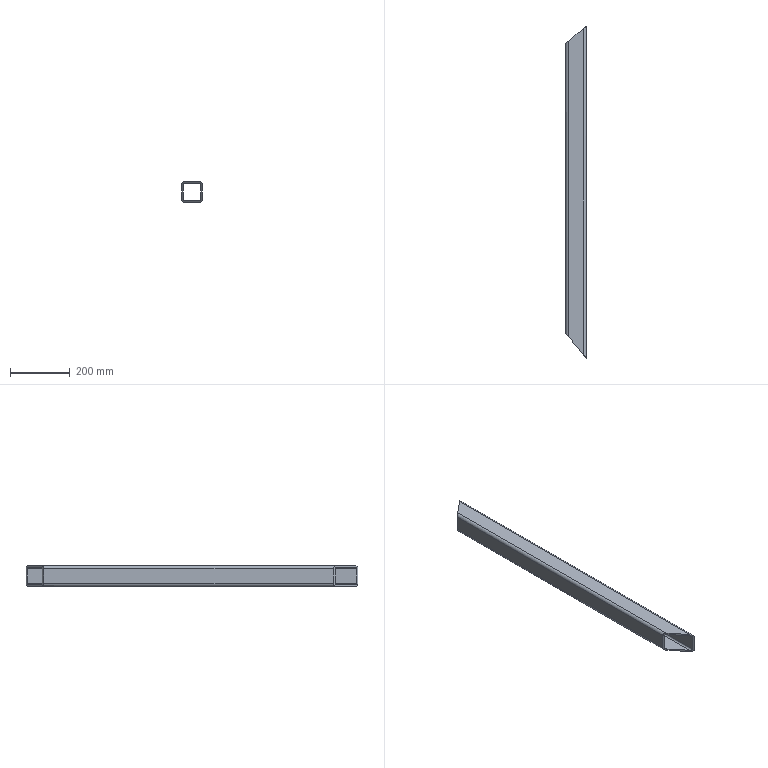Part | SolidWorks | features ICE 1, WeldMemberFeat 1, WeldmentFeature 1 | 1 solid | 18 faces | box 70 x 1116 x 70 mm | volume 1291200 mm3 | plane 10 | cylinder 8 | commonest cylinder face diameters 10 x4 20 x4
STEP:
#1=CARTESIAN_POINT('',(35.,0.,25.));
#2=VERTEX_POINT('',#1);
#3=CARTESIAN_POINT('',(35.,0.,-25.));
#4=VERTEX_POINT('',#3);
#5=CARTESIAN_POINT('',(35.,0.,-25.));
#6=DIRECTION('',(0.,0.,-1.));
#7=VECTOR('',#6,1000.);
#8=LINE('',#5,#7);
#9=EDGE_CURVE('',#2,#4,#8,.T.);
#10=ORIENTED_EDGE('',*,*,#9,.T.);
#11=CARTESIAN_POINT('',(35.,1116.,-25.));
#12=VERTEX_POINT('',#11);
#13=CARTESIAN_POINT('',(35.,1116.,-25.));
#14=DIRECTION('',(0.,-1.,0.));
#15=VECTOR('',#14,1000.);
#16=LINE('',#13,#15);
#17=EDGE_CURVE('',#12,#4,#16,.T.);
#18=ORIENTED_EDGE('',*,*,#17,.F.);
#19=CARTESIAN_POINT('',(35.,1116.,25.));
#20=VERTEX_POINT('',#19);
#21=CARTESIAN_POINT('',(35.,1116.,-25.));
#22=DIRECTION('',(0.,0.,-1.));
#23=VECTOR('',#22,1000.);
#24=LINE('',#21,#23);
#25=EDGE_CURVE('',#20,#12,#24,.T.);
#26=ORIENTED_EDGE('',*,*,#25,.F.);
#27=CARTESIAN_POINT('',(35.,1116.,25.));
#28=DIRECTION('',(0.,-1.,0.));
#29=VECTOR('',#28,1000.);
#30=LINE('',#27,#29);
#31=EDGE_CURVE('',#20,#2,#30,.T.);
#32=ORIENTED_EDGE('',*,*,#31,.T.);
#33=EDGE_LOOP('',(#10,#18,#26,#32));
#34=FACE_OUTER_BOUND('',#33,.T.);
#35=CARTESIAN_POINT('',(35.,1116.,-25.));
#36=DIRECTION('',(-1.,0.,0.));
#37=DIRECTION('',(0.,0.,1.));
#38=AXIS2_PLACEMENT_3D('',#35,#36,#37);
#39=PLANE('',#38);
#40=ADVANCED_FACE('',(#34),#39,.F.);
#41=CARTESIAN_POINT('',(-35.,1056.964,25.));
#42=VERTEX_POINT('',#41);
#43=CARTESIAN_POINT('',(-35.,83.,25.));
#44=VERTEX_POINT('',#43);
#45=CARTESIAN_POINT('',(-35.,1116.,25.));
#46=DIRECTION('',(0.,-1.,0.));
#47=VECTOR('',#46,1000.);
#48=LINE('',#45,#47);
#49=EDGE_CURVE('',#42,#44,#48,.T.);
#50=ORIENTED_EDGE('',*,*,#49,.F.);
#51=CARTESIAN_POINT('',(-35.,1056.964,-25.));
#52=VERTEX_POINT('',#51);
#53=CARTESIAN_POINT('',(-35.,1056.964,-35.));
#54=DIRECTION('',(0.,0.,1.));
#55=VECTOR('',#54,1000.);
#56=LINE('',#53,#55);
#57=EDGE_CURVE('',#52,#42,#56,.T.);
#58=ORIENTED_EDGE('',*,*,#57,.F.);
#59=CARTESIAN_POINT('',(-35.,83.,-25.));
#60=VERTEX_POINT('',#59);
#61=CARTESIAN_POINT('',(-35.,1116.,-25.));
#62=DIRECTION('',(0.,-1.,0.));
#63=VECTOR('',#62,1000.);
#64=LINE('',#61,#63);
#65=EDGE_CURVE('',#52,#60,#64,.T.);
#66=ORIENTED_EDGE('',*,*,#65,.T.);
#67=CARTESIAN_POINT('',(-35.,83.,-35.));
#68=DIRECTION('',(0.,0.,1.));
#69=VECTOR('',#68,1000.);
#70=LINE('',#67,#69);
#71=EDGE_CURVE('',#60,#44,#70,.T.);
#72=ORIENTED_EDGE('',*,*,#71,.T.);
#73=EDGE_LOOP('',(#50,#58,#66,#72));
#74=FACE_OUTER_BOUND('',#73,.T.);
#75=CARTESIAN_POINT('',(-35.,1116.,25.));
#76=DIRECTION('',(1.,0.,0.));
#77=DIRECTION('',(0.,0.,-1.));
#78=AXIS2_PLACEMENT_3D('',#75,#76,#77);
#79=PLANE('',#78);
#80=ADVANCED_FACE('',(#74),#79,.F.);
#81=ORIENTED_EDGE('',*,*,#65,.F.);
#82=CARTESIAN_POINT('',(-25.,1065.398,-35.));
#83=VERTEX_POINT('',#82);
#84=CARTESIAN_POINT('',(-35.,1056.964,-25.));
#85=CARTESIAN_POINT('',(-35.,1056.964,-30.858));
#86=CARTESIAN_POINT('',(-30.858,1060.457,-35.));
#87=CARTESIAN_POINT('',(-25.,1065.398,-35.));
#88=(BOUNDED_CURVE()B_SPLINE_CURVE(3,(#84,#85,#86,#87),.UNSPECIFIED.,.F.,.F.)B_SPLINE_CURVE_WITH_KNOTS((4,4),(0.,1.571),.UNSPECIFIED.)CURVE()GEOMETRIC_REPRESENTATION_ITEM()RATIONAL_B_SPLINE_CURVE((1.,0.8047,0.8047,1.))REPRESENTATION_ITEM(''));
#89=EDGE_CURVE('',#52,#83,#88,.T.);
#90=ORIENTED_EDGE('',*,*,#89,.T.);
#91=CARTESIAN_POINT('',(-25.,71.143,-35.));
#92=VERTEX_POINT('',#91);
#93=CARTESIAN_POINT('',(-25.,1116.,-35.));
#94=DIRECTION('',(0.,-1.,0.));
#95=VECTOR('',#94,1000.);
#96=LINE('',#93,#95);
#97=EDGE_CURVE('',#83,#92,#96,.T.);
#98=ORIENTED_EDGE('',*,*,#97,.T.);
#99=CARTESIAN_POINT('',(-25.,71.143,-35.));
#100=CARTESIAN_POINT('',(-30.858,78.089,-35.));
#101=CARTESIAN_POINT('',(-35.,83.,-30.858));
#102=CARTESIAN_POINT('',(-35.,83.,-25.));
#103=(BOUNDED_CURVE()B_SPLINE_CURVE(3,(#99,#100,#101,#102),.UNSPECIFIED.,.F.,.F.)B_SPLINE_CURVE_WITH_KNOTS((4,4),(1.571,3.142),.UNSPECIFIED.)CURVE()GEOMETRIC_REPRESENTATION_ITEM()RATIONAL_B_SPLINE_CURVE((1.,0.8047,0.8047,1.))REPRESENTATION_ITEM(''));
#104=EDGE_CURVE('',#92,#60,#103,.T.);
#105=ORIENTED_EDGE('',*,*,#104,.T.);
#106=EDGE_LOOP('',(#81,#90,#98,#105));
#107=FACE_OUTER_BOUND('',#106,.T.);
#108=CARTESIAN_POINT('',(-25.,1116.,-25.));
#109=DIRECTION('',(0.,-1.,0.));
#110=DIRECTION('',(0.,0.,-1.));
#111=AXIS2_PLACEMENT_3D('',#108,#109,#110);
#112=CYLINDRICAL_SURFACE('',#111,10.);
#113=ADVANCED_FACE('',(#107),#112,.T.);
#114=ORIENTED_EDGE('',*,*,#97,.F.);
#115=CARTESIAN_POINT('',(25.,1107.566,-35.));
#116=VERTEX_POINT('',#115);
#117=CARTESIAN_POINT('',(35.,1116.,-35.));
#118=DIRECTION('',(0.7644,0.6447,0.));
#119=VECTOR('',#118,1000.);
#120=LINE('',#117,#119);
#121=EDGE_CURVE('',#83,#116,#120,.T.);
#122=ORIENTED_EDGE('',*,*,#121,.T.);
#123=CARTESIAN_POINT('',(25.,11.857,-35.));
#124=VERTEX_POINT('',#123);
#125=CARTESIAN_POINT('',(25.,1116.,-35.));
#126=DIRECTION('',(0.,-1.,0.));
#127=VECTOR('',#126,1000.);
#128=LINE('',#125,#127);
#129=EDGE_CURVE('',#116,#124,#128,.T.);
#130=ORIENTED_EDGE('',*,*,#129,.T.);
#131=CARTESIAN_POINT('',(-35.,83.,-35.));
#132=DIRECTION('',(-0.6447,0.7644,0.));
#133=VECTOR('',#132,1000.);
#134=LINE('',#131,#133);
#135=EDGE_CURVE('',#124,#92,#134,.T.);
#136=ORIENTED_EDGE('',*,*,#135,.T.);
#137=EDGE_LOOP('',(#114,#122,#130,#136));
#138=FACE_OUTER_BOUND('',#137,.T.);
#139=CARTESIAN_POINT('',(25.,1116.,-35.));
#140=DIRECTION('',(0.,0.,1.));
#141=DIRECTION('',(1.,0.,0.));
#142=AXIS2_PLACEMENT_3D('',#139,#140,#141);
#143=PLANE('',#142);
#144=ADVANCED_FACE('',(#138),#143,.F.);
#145=ORIENTED_EDGE('',*,*,#129,.F.);
#146=CARTESIAN_POINT('',(25.,1107.566,-35.));
#147=CARTESIAN_POINT('',(30.858,1112.507,-35.));
#148=CARTESIAN_POINT('',(35.,1116.,-30.858));
#149=CARTESIAN_POINT('',(35.,1116.,-25.));
#150=(BOUNDED_CURVE()B_SPLINE_CURVE(3,(#146,#147,#148,#149),.UNSPECIFIED.,.F.,.F.)B_SPLINE_CURVE_WITH_KNOTS((4,4),(1.571,3.142),.UNSPECIFIED.)CURVE()GEOMETRIC_REPRESENTATION_ITEM()RATIONAL_B_SPLINE_CURVE((1.,0.8047,0.8047,1.))REPRESENTATION_ITEM(''));
#151=EDGE_CURVE('',#116,#12,#150,.T.);
#152=ORIENTED_EDGE('',*,*,#151,.T.);
#153=ORIENTED_EDGE('',*,*,#17,.T.);
#154=CARTESIAN_POINT('',(35.,0.,-25.));
#155=CARTESIAN_POINT('',(35.,0.,-30.858));
#156=CARTESIAN_POINT('',(30.858,4.911,-35.));
#157=CARTESIAN_POINT('',(25.,11.857,-35.));
#158=(BOUNDED_CURVE()B_SPLINE_CURVE(3,(#154,#155,#156,#157),.UNSPECIFIED.,.F.,.F.)B_SPLINE_CURVE_WITH_KNOTS((4,4),(0.,1.571),.UNSPECIFIED.)CURVE()GEOMETRIC_REPRESENTATION_ITEM()RATIONAL_B_SPLINE_CURVE((1.,0.8047,0.8047,1.))REPRESENTATION_ITEM(''));
#159=EDGE_CURVE('',#4,#124,#158,.T.);
#160=ORIENTED_EDGE('',*,*,#159,.T.);
#161=EDGE_LOOP('',(#145,#152,#153,#160));
#162=FACE_OUTER_BOUND('',#161,.T.);
#163=CARTESIAN_POINT('',(25.,1116.,-25.));
#164=DIRECTION('',(0.,-1.,0.));
#165=DIRECTION('',(0.,0.,-1.));
#166=AXIS2_PLACEMENT_3D('',#163,#164,#165);
#167=CYLINDRICAL_SURFACE('',#166,10.);
#168=ADVANCED_FACE('',(#162),#167,.T.);
#169=ORIENTED_EDGE('',*,*,#31,.F.);
#170=CARTESIAN_POINT('',(25.,1107.566,35.));
#171=VERTEX_POINT('',#170);
#172=CARTESIAN_POINT('',(35.,1116.,25.));
#173=CARTESIAN_POINT('',(35.,1116.,30.858));
#174=CARTESIAN_POINT('',(30.858,1112.507,35.));
#175=CARTESIAN_POINT('',(25.,1107.566,35.));
#176=(BOUNDED_CURVE()B_SPLINE_CURVE(3,(#172,#173,#174,#175),.UNSPECIFIED.,.F.,.F.)B_SPLINE_CURVE_WITH_KNOTS((4,4),(3.142,4.712),.UNSPECIFIED.)CURVE()GEOMETRIC_REPRESENTATION_ITEM()RATIONAL_B_SPLINE_CURVE((1.,0.8047,0.8047,1.))REPRESENTATION_ITEM(''));
#177=EDGE_CURVE('',#20,#171,#176,.T.);
#178=ORIENTED_EDGE('',*,*,#177,.T.);
#179=CARTESIAN_POINT('',(25.,11.857,35.));
#180=VERTEX_POINT('',#179);
#181=CARTESIAN_POINT('',(25.,1116.,35.));
#182=DIRECTION('',(0.,-1.,0.));
#183=VECTOR('',#182,1000.);
#184=LINE('',#181,#183);
#185=EDGE_CURVE('',#171,#180,#184,.T.);
#186=ORIENTED_EDGE('',*,*,#185,.T.);
#187=CARTESIAN_POINT('',(25.,11.857,35.));
#188=CARTESIAN_POINT('',(30.858,4.911,35.));
#189=CARTESIAN_POINT('',(35.,0.,30.858));
#190=CARTESIAN_POINT('',(35.,0.,25.));
#191=(BOUNDED_CURVE()B_SPLINE_CURVE(3,(#187,#188,#189,#190),.UNSPECIFIED.,.F.,.F.)B_SPLINE_CURVE_WITH_KNOTS((4,4),(4.712,6.283),.UNSPECIFIED.)CURVE()GEOMETRIC_REPRESENTATION_ITEM()RATIONAL_B_SPLINE_CURVE((1.,0.8047,0.8047,1.))REPRESENTATION_ITEM(''));
#192=EDGE_CURVE('',#180,#2,#191,.T.);
#193=ORIENTED_EDGE('',*,*,#192,.T.);
#194=EDGE_LOOP('',(#169,#178,#186,#193));
#195=FACE_OUTER_BOUND('',#194,.T.);
#196=CARTESIAN_POINT('',(25.,1116.,25.));
#197=DIRECTION('',(0.,-1.,0.));
#198=DIRECTION('',(0.,0.,-1.));
#199=AXIS2_PLACEMENT_3D('',#196,#197,#198);
#200=CYLINDRICAL_SURFACE('',#199,10.);
#201=ADVANCED_FACE('',(#195),#200,.T.);
#202=ORIENTED_EDGE('',*,*,#185,.F.);
#203=CARTESIAN_POINT('',(-25.,1065.398,35.));
#204=VERTEX_POINT('',#203);
#205=CARTESIAN_POINT('',(-0.0615,1086.43,35.));
#206=DIRECTION('',(-0.7644,-0.6447,0.));
#207=VECTOR('',#206,1000.);
#208=LINE('',#205,#207);
#209=EDGE_CURVE('',#171,#204,#208,.T.);
#210=ORIENTED_EDGE('',*,*,#209,.T.);
#211=CARTESIAN_POINT('',(-25.,71.143,35.));
#212=VERTEX_POINT('',#211);
#213=CARTESIAN_POINT('',(-25.,1116.,35.));
#214=DIRECTION('',(0.,-1.,0.));
#215=VECTOR('',#214,1000.);
#216=LINE('',#213,#215);
#217=EDGE_CURVE('',#204,#212,#216,.T.);
#218=ORIENTED_EDGE('',*,*,#217,.T.);
#219=CARTESIAN_POINT('',(-539.939,681.714,35.));
#220=DIRECTION('',(0.6447,-0.7644,0.));
#221=VECTOR('',#220,1000.);
#222=LINE('',#219,#221);
#223=EDGE_CURVE('',#212,#180,#222,.T.);
#224=ORIENTED_EDGE('',*,*,#223,.T.);
#225=EDGE_LOOP('',(#202,#210,#218,#224));
#226=FACE_OUTER_BOUND('',#225,.T.);
#227=CARTESIAN_POINT('',(-25.,1116.,35.));
#228=DIRECTION('',(0.,0.,-1.));
#229=DIRECTION('',(-1.,0.,0.));
#230=AXIS2_PLACEMENT_3D('',#227,#228,#229);
#231=PLANE('',#230);
#232=ADVANCED_FACE('',(#226),#231,.F.);
#233=ORIENTED_EDGE('',*,*,#217,.F.);
#234=CARTESIAN_POINT('',(-25.,1065.398,35.));
#235=CARTESIAN_POINT('',(-30.858,1060.457,35.));
#236=CARTESIAN_POINT('',(-35.,1056.964,30.858));
#237=CARTESIAN_POINT('',(-35.,1056.964,25.));
#238=(BOUNDED_CURVE()B_SPLINE_CURVE(3,(#234,#235,#236,#237),.UNSPECIFIED.,.F.,.F.)B_SPLINE_CURVE_WITH_KNOTS((4,4),(4.712,6.283),.UNSPECIFIED.)CURVE()GEOMETRIC_REPRESENTATION_ITEM()RATIONAL_B_SPLINE_CURVE((1.,0.8047,0.8047,1.))REPRESENTATION_ITEM(''));
#239=EDGE_CURVE('',#204,#42,#238,.T.);
#240=ORIENTED_EDGE('',*,*,#239,.T.);
#241=ORIENTED_EDGE('',*,*,#49,.T.);
#242=CARTESIAN_POINT('',(-35.,83.,25.));
#243=CARTESIAN_POINT('',(-35.,83.,30.858));
#244=CARTESIAN_POINT('',(-30.858,78.089,35.));
#245=CARTESIAN_POINT('',(-25.,71.143,35.));
#246=(BOUNDED_CURVE()B_SPLINE_CURVE(3,(#242,#243,#244,#245),.UNSPECIFIED.,.F.,.F.)B_SPLINE_CURVE_WITH_KNOTS((4,4),(3.142,4.712),.UNSPECIFIED.)CURVE()GEOMETRIC_REPRESENTATION_ITEM()RATIONAL_B_SPLINE_CURVE((1.,0.8047,0.8047,1.))REPRESENTATION_ITEM(''));
#247=EDGE_CURVE('',#44,#212,#246,.T.);
#248=ORIENTED_EDGE('',*,*,#247,.T.);
#249=EDGE_LOOP('',(#233,#240,#241,#248));
#250=FACE_OUTER_BOUND('',#249,.T.);
#251=CARTESIAN_POINT('',(-25.,1116.,25.));
#252=DIRECTION('',(0.,-1.,0.));
#253=DIRECTION('',(0.,0.,-1.));
#254=AXIS2_PLACEMENT_3D('',#251,#252,#253);
#255=CYLINDRICAL_SURFACE('',#254,10.);
#256=ADVANCED_FACE('',(#250),#255,.T.);
#257=CARTESIAN_POINT('',(25.,11.857,30.));
#258=VERTEX_POINT('',#257);
#259=CARTESIAN_POINT('',(30.,5.929,25.));
#260=VERTEX_POINT('',#259);
#261=CARTESIAN_POINT('',(25.,11.857,30.));
#262=CARTESIAN_POINT('',(27.929,8.384,30.));
#263=CARTESIAN_POINT('',(30.,5.929,27.929));
#264=CARTESIAN_POINT('',(30.,5.929,25.));
#265=(BOUNDED_CURVE()B_SPLINE_CURVE(3,(#261,#262,#263,#264),.UNSPECIFIED.,.F.,.T.)B_SPLINE_CURVE_WITH_KNOTS((4,4),(4.712,6.283),.UNSPECIFIED.)CURVE()GEOMETRIC_REPRESENTATION_ITEM()RATIONAL_B_SPLINE_CURVE((1.,0.8047,0.8047,1.))REPRESENTATION_ITEM(''));
#266=EDGE_CURVE('',#258,#260,#265,.T.);
#267=ORIENTED_EDGE('',*,*,#266,.T.);
#268=CARTESIAN_POINT('',(30.,5.929,-25.));
#269=VERTEX_POINT('',#268);
#270=CARTESIAN_POINT('',(30.,5.929,-25.));
#271=DIRECTION('',(0.,0.,-1.));
#272=VECTOR('',#271,1000.);
#273=LINE('',#270,#272);
#274=EDGE_CURVE('',#260,#269,#273,.T.);
#275=ORIENTED_EDGE('',*,*,#274,.T.);
#276=CARTESIAN_POINT('',(25.,11.857,-30.));
#277=VERTEX_POINT('',#276);
#278=CARTESIAN_POINT('',(30.,5.929,-25.));
#279=CARTESIAN_POINT('',(30.,5.929,-27.929));
#280=CARTESIAN_POINT('',(27.929,8.384,-30.));
#281=CARTESIAN_POINT('',(25.,11.857,-30.));
#282=(BOUNDED_CURVE()B_SPLINE_CURVE(3,(#278,#279,#280,#281),.UNSPECIFIED.,.F.,.F.)B_SPLINE_CURVE_WITH_KNOTS((4,4),(0.,1.571),.UNSPECIFIED.)CURVE()GEOMETRIC_REPRESENTATION_ITEM()RATIONAL_B_SPLINE_CURVE((1.,0.8047,0.8047,1.))REPRESENTATION_ITEM(''));
#283=EDGE_CURVE('',#269,#277,#282,.T.);
#284=ORIENTED_EDGE('',*,*,#283,.T.);
#285=CARTESIAN_POINT('',(-25.,71.143,-30.));
#286=VERTEX_POINT('',#285);
#287=CARTESIAN_POINT('',(-519.157,657.072,-30.));
#288=DIRECTION('',(-0.6447,0.7644,0.));
#289=VECTOR('',#288,1000.);
#290=LINE('',#287,#289);
#291=EDGE_CURVE('',#277,#286,#290,.T.);
#292=ORIENTED_EDGE('',*,*,#291,.T.);
#293=CARTESIAN_POINT('',(-30.,77.071,-25.));
#294=VERTEX_POINT('',#293);
#295=CARTESIAN_POINT('',(-25.,71.143,-30.));
#296=CARTESIAN_POINT('',(-27.929,74.616,-30.));
#297=CARTESIAN_POINT('',(-30.,77.071,-27.929));
#298=CARTESIAN_POINT('',(-30.,77.071,-25.));
#299=(BOUNDED_CURVE()B_SPLINE_CURVE(3,(#295,#296,#297,#298),.UNSPECIFIED.,.F.,.F.)B_SPLINE_CURVE_WITH_KNOTS((4,4),(1.571,3.142),.UNSPECIFIED.)CURVE()GEOMETRIC_REPRESENTATION_ITEM()RATIONAL_B_SPLINE_CURVE((1.,0.8047,0.8047,1.))REPRESENTATION_ITEM(''));
#300=EDGE_CURVE('',#286,#294,#299,.T.);
#301=ORIENTED_EDGE('',*,*,#300,.T.);
#302=CARTESIAN_POINT('',(-30.,77.071,25.));
#303=VERTEX_POINT('',#302);
#304=CARTESIAN_POINT('',(-30.,77.071,25.));
#305=DIRECTION('',(0.,0.,1.));
#306=VECTOR('',#305,1000.);
#307=LINE('',#304,#306);
#308=EDGE_CURVE('',#294,#303,#307,.T.);
#309=ORIENTED_EDGE('',*,*,#308,.T.);
#310=CARTESIAN_POINT('',(-25.,71.143,30.));
#311=VERTEX_POINT('',#310);
#312=CARTESIAN_POINT('',(-30.,77.071,25.));
#313=CARTESIAN_POINT('',(-30.,77.071,27.929));
#314=CARTESIAN_POINT('',(-27.929,74.616,30.));
#315=CARTESIAN_POINT('',(-25.,71.143,30.));
#316=(BOUNDED_CURVE()B_SPLINE_CURVE(3,(#312,#313,#314,#315),.UNSPECIFIED.,.F.,.F.)B_SPLINE_CURVE_WITH_KNOTS((4,4),(3.142,4.712),.UNSPECIFIED.)CURVE()GEOMETRIC_REPRESENTATION_ITEM()RATIONAL_B_SPLINE_CURVE((1.,0.8047,0.8047,1.))REPRESENTATION_ITEM(''));
#317=EDGE_CURVE('',#303,#311,#316,.T.);
#318=ORIENTED_EDGE('',*,*,#317,.T.);
#319=CARTESIAN_POINT('',(-539.939,681.714,30.));
#320=DIRECTION('',(0.6447,-0.7644,0.));
#321=VECTOR('',#320,1000.);
#322=LINE('',#319,#321);
#323=EDGE_CURVE('',#311,#258,#322,.T.);
#324=ORIENTED_EDGE('',*,*,#323,.T.);
#325=EDGE_LOOP('',(#267,#275,#284,#292,#301,#309,#318,#324));
#326=FACE_BOUND('',#325,.T.);
#327=ORIENTED_EDGE('',*,*,#71,.F.);
#328=ORIENTED_EDGE('',*,*,#104,.F.);
#329=ORIENTED_EDGE('',*,*,#135,.F.);
#330=ORIENTED_EDGE('',*,*,#159,.F.);
#331=ORIENTED_EDGE('',*,*,#9,.F.);
#332=ORIENTED_EDGE('',*,*,#192,.F.);
#333=ORIENTED_EDGE('',*,*,#223,.F.);
#334=ORIENTED_EDGE('',*,*,#247,.F.);
#335=EDGE_LOOP('',(#327,#328,#329,#330,#331,#332,#333,#334));
#336=FACE_OUTER_BOUND('',#335,.T.);
#337=CARTESIAN_POINT('',(-35.,83.,-35.));
#338=DIRECTION('',(0.7644,0.6447,0.));
#339=DIRECTION('',(-0.6447,0.7644,0.));
#340=AXIS2_PLACEMENT_3D('',#337,#338,#339);
#341=PLANE('',#340);
#342=ADVANCED_FACE('',(#326,#336),#341,.F.);
#343=CARTESIAN_POINT('',(30.,1111.783,25.));
#344=VERTEX_POINT('',#343);
#345=CARTESIAN_POINT('',(25.,1107.566,30.));
#346=VERTEX_POINT('',#345);
#347=CARTESIAN_POINT('',(30.,1111.783,25.));
#348=CARTESIAN_POINT('',(30.,1111.783,27.929));
#349=CARTESIAN_POINT('',(27.929,1110.036,30.));
#350=CARTESIAN_POINT('',(25.,1107.566,30.));
#351=(BOUNDED_CURVE()B_SPLINE_CURVE(3,(#347,#348,#349,#350),.UNSPECIFIED.,.F.,.F.)B_SPLINE_CURVE_WITH_KNOTS((4,4),(3.142,4.712),.UNSPECIFIED.)CURVE()GEOMETRIC_REPRESENTATION_ITEM()RATIONAL_B_SPLINE_CURVE((1.,0.8047,0.8047,1.))REPRESENTATION_ITEM(''));
#352=EDGE_CURVE('',#344,#346,#351,.T.);
#353=ORIENTED_EDGE('',*,*,#352,.T.);
#354=CARTESIAN_POINT('',(-25.,1065.398,30.));
#355=VERTEX_POINT('',#354);
#356=CARTESIAN_POINT('',(-0.0615,1086.43,30.));
#357=DIRECTION('',(-0.7644,-0.6447,0.));
#358=VECTOR('',#357,1000.);
#359=LINE('',#356,#358);
#360=EDGE_CURVE('',#346,#355,#359,.T.);
#361=ORIENTED_EDGE('',*,*,#360,.T.);
#362=CARTESIAN_POINT('',(-30.,1061.181,25.));
#363=VERTEX_POINT('',#362);
#364=CARTESIAN_POINT('',(-25.,1065.398,30.));
#365=CARTESIAN_POINT('',(-27.929,1062.927,30.));
#366=CARTESIAN_POINT('',(-30.,1061.181,27.929));
#367=CARTESIAN_POINT('',(-30.,1061.181,25.));
#368=(BOUNDED_CURVE()B_SPLINE_CURVE(3,(#364,#365,#366,#367),.UNSPECIFIED.,.F.,.F.)B_SPLINE_CURVE_WITH_KNOTS((4,4),(4.712,6.283),.UNSPECIFIED.)CURVE()GEOMETRIC_REPRESENTATION_ITEM()RATIONAL_B_SPLINE_CURVE((1.,0.8047,0.8047,1.))REPRESENTATION_ITEM(''));
#369=EDGE_CURVE('',#355,#363,#368,.T.);
#370=ORIENTED_EDGE('',*,*,#369,.T.);
#371=CARTESIAN_POINT('',(-30.,1061.181,-25.));
#372=VERTEX_POINT('',#371);
#373=CARTESIAN_POINT('',(-30.,1061.181,25.));
#374=DIRECTION('',(0.,0.,-1.));
#375=VECTOR('',#374,1000.);
#376=LINE('',#373,#375);
#377=EDGE_CURVE('',#363,#372,#376,.T.);
#378=ORIENTED_EDGE('',*,*,#377,.T.);
#379=CARTESIAN_POINT('',(-25.,1065.398,-30.));
#380=VERTEX_POINT('',#379);
#381=CARTESIAN_POINT('',(-30.,1061.181,-25.));
#382=CARTESIAN_POINT('',(-30.,1061.181,-27.929));
#383=CARTESIAN_POINT('',(-27.929,1062.927,-30.));
#384=CARTESIAN_POINT('',(-25.,1065.398,-30.));
#385=(BOUNDED_CURVE()B_SPLINE_CURVE(3,(#381,#382,#383,#384),.UNSPECIFIED.,.F.,.T.)B_SPLINE_CURVE_WITH_KNOTS((4,4),(0.,1.571),.UNSPECIFIED.)CURVE()GEOMETRIC_REPRESENTATION_ITEM()RATIONAL_B_SPLINE_CURVE((1.,0.8047,0.8047,1.))REPRESENTATION_ITEM(''));
#386=EDGE_CURVE('',#372,#380,#385,.T.);
#387=ORIENTED_EDGE('',*,*,#386,.T.);
#388=CARTESIAN_POINT('',(25.,1107.566,-30.));
#389=VERTEX_POINT('',#388);
#390=CARTESIAN_POINT('',(29.156,1111.072,-30.));
#391=DIRECTION('',(0.7644,0.6447,0.));
#392=VECTOR('',#391,1000.);
#393=LINE('',#390,#392);
#394=EDGE_CURVE('',#380,#389,#393,.T.);
#395=ORIENTED_EDGE('',*,*,#394,.T.);
#396=CARTESIAN_POINT('',(30.,1111.783,-25.));
#397=VERTEX_POINT('',#396);
#398=CARTESIAN_POINT('',(25.,1107.566,-30.));
#399=CARTESIAN_POINT('',(27.929,1110.036,-30.));
#400=CARTESIAN_POINT('',(30.,1111.783,-27.929));
#401=CARTESIAN_POINT('',(30.,1111.783,-25.));
#402=(BOUNDED_CURVE()B_SPLINE_CURVE(3,(#398,#399,#400,#401),.UNSPECIFIED.,.F.,.T.)B_SPLINE_CURVE_WITH_KNOTS((4,4),(1.571,3.142),.UNSPECIFIED.)CURVE()GEOMETRIC_REPRESENTATION_ITEM()RATIONAL_B_SPLINE_CURVE((1.,0.8047,0.8047,1.))REPRESENTATION_ITEM(''));
#403=EDGE_CURVE('',#389,#397,#402,.T.);
#404=ORIENTED_EDGE('',*,*,#403,.T.);
#405=CARTESIAN_POINT('',(30.,1111.783,-25.));
#406=DIRECTION('',(0.,0.,1.));
#407=VECTOR('',#406,1000.);
#408=LINE('',#405,#407);
#409=EDGE_CURVE('',#397,#344,#408,.T.);
#410=ORIENTED_EDGE('',*,*,#409,.T.);
#411=EDGE_LOOP('',(#353,#361,#370,#378,#387,#395,#404,#410));
#412=FACE_BOUND('',#411,.T.);
#413=ORIENTED_EDGE('',*,*,#209,.F.);
#414=ORIENTED_EDGE('',*,*,#177,.F.);
#415=ORIENTED_EDGE('',*,*,#25,.T.);
#416=ORIENTED_EDGE('',*,*,#151,.F.);
#417=ORIENTED_EDGE('',*,*,#121,.F.);
#418=ORIENTED_EDGE('',*,*,#89,.F.);
#419=ORIENTED_EDGE('',*,*,#57,.T.);
#420=ORIENTED_EDGE('',*,*,#239,.F.);
#421=EDGE_LOOP('',(#413,#414,#415,#416,#417,#418,#419,#420));
#422=FACE_OUTER_BOUND('',#421,.T.);
#423=CARTESIAN_POINT('',(35.,1116.,-35.));
#424=DIRECTION('',(0.6447,-0.7644,0.));
#425=DIRECTION('',(0.7644,0.6447,0.));
#426=AXIS2_PLACEMENT_3D('',#423,#424,#425);
#427=PLANE('',#426);
#428=ADVANCED_FACE('',(#412,#422),#427,.F.);
#429=ORIENTED_EDGE('',*,*,#352,.F.);
#430=CARTESIAN_POINT('',(30.,1116.,25.));
#431=DIRECTION('',(0.,-1.,0.));
#432=VECTOR('',#431,1000.);
#433=LINE('',#430,#432);
#434=EDGE_CURVE('',#344,#260,#433,.T.);
#435=ORIENTED_EDGE('',*,*,#434,.T.);
#436=ORIENTED_EDGE('',*,*,#266,.F.);
#437=CARTESIAN_POINT('',(25.,1116.,30.));
#438=DIRECTION('',(0.,-1.,0.));
#439=VECTOR('',#438,1000.);
#440=LINE('',#437,#439);
#441=EDGE_CURVE('',#346,#258,#440,.T.);
#442=ORIENTED_EDGE('',*,*,#441,.F.);
#443=EDGE_LOOP('',(#429,#435,#436,#442));
#444=FACE_OUTER_BOUND('',#443,.T.);
#445=CARTESIAN_POINT('',(25.,1116.,25.));
#446=DIRECTION('',(0.,-1.,0.));
#447=DIRECTION('',(0.,0.,-1.));
#448=AXIS2_PLACEMENT_3D('',#445,#446,#447);
#449=CYLINDRICAL_SURFACE('',#448,5.);
#450=ADVANCED_FACE('',(#444),#449,.F.);
#451=ORIENTED_EDGE('',*,*,#360,.F.);
#452=ORIENTED_EDGE('',*,*,#441,.T.);
#453=ORIENTED_EDGE('',*,*,#323,.F.);
#454=CARTESIAN_POINT('',(-25.,1116.,30.));
#455=DIRECTION('',(0.,-1.,0.));
#456=VECTOR('',#455,1000.);
#457=LINE('',#454,#456);
#458=EDGE_CURVE('',#355,#311,#457,.T.);
#459=ORIENTED_EDGE('',*,*,#458,.F.);
#460=EDGE_LOOP('',(#451,#452,#453,#459));
#461=FACE_OUTER_BOUND('',#460,.T.);
#462=CARTESIAN_POINT('',(-25.,1116.,30.));
#463=DIRECTION('',(0.,0.,-1.));
#464=DIRECTION('',(-1.,0.,0.));
#465=AXIS2_PLACEMENT_3D('',#462,#463,#464);
#466=PLANE('',#465);
#467=ADVANCED_FACE('',(#461),#466,.T.);
#468=ORIENTED_EDGE('',*,*,#369,.F.);
#469=ORIENTED_EDGE('',*,*,#458,.T.);
#470=ORIENTED_EDGE('',*,*,#317,.F.);
#471=CARTESIAN_POINT('',(-30.,1116.,25.));
#472=DIRECTION('',(0.,-1.,0.));
#473=VECTOR('',#472,1000.);
#474=LINE('',#471,#473);
#475=EDGE_CURVE('',#363,#303,#474,.T.);
#476=ORIENTED_EDGE('',*,*,#475,.F.);
#477=EDGE_LOOP('',(#468,#469,#470,#476));
#478=FACE_OUTER_BOUND('',#477,.T.);
#479=CARTESIAN_POINT('',(-25.,1116.,25.));
#480=DIRECTION('',(0.,-1.,0.));
#481=DIRECTION('',(0.,0.,-1.));
#482=AXIS2_PLACEMENT_3D('',#479,#480,#481);
#483=CYLINDRICAL_SURFACE('',#482,5.);
#484=ADVANCED_FACE('',(#478),#483,.F.);
#485=ORIENTED_EDGE('',*,*,#377,.F.);
#486=ORIENTED_EDGE('',*,*,#475,.T.);
#487=ORIENTED_EDGE('',*,*,#308,.F.);
#488=CARTESIAN_POINT('',(-30.,1116.,-25.));
#489=DIRECTION('',(0.,-1.,0.));
#490=VECTOR('',#489,1000.);
#491=LINE('',#488,#490);
#492=EDGE_CURVE('',#372,#294,#491,.T.);
#493=ORIENTED_EDGE('',*,*,#492,.F.);
#494=EDGE_LOOP('',(#485,#486,#487,#493));
#495=FACE_OUTER_BOUND('',#494,.T.);
#496=CARTESIAN_POINT('',(-30.,1116.,25.));
#497=DIRECTION('',(1.,0.,0.));
#498=DIRECTION('',(0.,0.,-1.));
#499=AXIS2_PLACEMENT_3D('',#496,#497,#498);
#500=PLANE('',#499);
#501=ADVANCED_FACE('',(#495),#500,.T.);
#502=ORIENTED_EDGE('',*,*,#386,.F.);
#503=ORIENTED_EDGE('',*,*,#492,.T.);
#504=ORIENTED_EDGE('',*,*,#300,.F.);
#505=CARTESIAN_POINT('',(-25.,1116.,-30.));
#506=DIRECTION('',(0.,-1.,0.));
#507=VECTOR('',#506,1000.);
#508=LINE('',#505,#507);
#509=EDGE_CURVE('',#380,#286,#508,.T.);
#510=ORIENTED_EDGE('',*,*,#509,.F.);
#511=EDGE_LOOP('',(#502,#503,#504,#510));
#512=FACE_OUTER_BOUND('',#511,.T.);
#513=CARTESIAN_POINT('',(-25.,1116.,-25.));
#514=DIRECTION('',(0.,-1.,0.));
#515=DIRECTION('',(0.,0.,-1.));
#516=AXIS2_PLACEMENT_3D('',#513,#514,#515);
#517=CYLINDRICAL_SURFACE('',#516,5.);
#518=ADVANCED_FACE('',(#512),#517,.F.);
#519=ORIENTED_EDGE('',*,*,#394,.F.);
#520=ORIENTED_EDGE('',*,*,#509,.T.);
#521=ORIENTED_EDGE('',*,*,#291,.F.);
#522=CARTESIAN_POINT('',(25.,1116.,-30.));
#523=DIRECTION('',(0.,-1.,0.));
#524=VECTOR('',#523,1000.);
#525=LINE('',#522,#524);
#526=EDGE_CURVE('',#389,#277,#525,.T.);
#527=ORIENTED_EDGE('',*,*,#526,.F.);
#528=EDGE_LOOP('',(#519,#520,#521,#527));
#529=FACE_OUTER_BOUND('',#528,.T.);
#530=CARTESIAN_POINT('',(25.,1116.,-30.));
#531=DIRECTION('',(0.,0.,1.));
#532=DIRECTION('',(1.,0.,0.));
#533=AXIS2_PLACEMENT_3D('',#530,#531,#532);
#534=PLANE('',#533);
#535=ADVANCED_FACE('',(#529),#534,.T.);
#536=ORIENTED_EDGE('',*,*,#403,.F.);
#537=ORIENTED_EDGE('',*,*,#526,.T.);
#538=ORIENTED_EDGE('',*,*,#283,.F.);
#539=CARTESIAN_POINT('',(30.,1116.,-25.));
#540=DIRECTION('',(0.,-1.,0.));
#541=VECTOR('',#540,1000.);
#542=LINE('',#539,#541);
#543=EDGE_CURVE('',#397,#269,#542,.T.);
#544=ORIENTED_EDGE('',*,*,#543,.F.);
#545=EDGE_LOOP('',(#536,#537,#538,#544));
#546=FACE_OUTER_BOUND('',#545,.T.);
#547=CARTESIAN_POINT('',(25.,1116.,-25.));
#548=DIRECTION('',(0.,-1.,0.));
#549=DIRECTION('',(0.,0.,-1.));
#550=AXIS2_PLACEMENT_3D('',#547,#548,#549);
#551=CYLINDRICAL_SURFACE('',#550,5.);
#552=ADVANCED_FACE('',(#546),#551,.F.);
#553=ORIENTED_EDGE('',*,*,#409,.F.);
#554=ORIENTED_EDGE('',*,*,#543,.T.);
#555=ORIENTED_EDGE('',*,*,#274,.F.);
#556=ORIENTED_EDGE('',*,*,#434,.F.);
#557=EDGE_LOOP('',(#553,#554,#555,#556));
#558=FACE_OUTER_BOUND('',#557,.T.);
#559=CARTESIAN_POINT('',(30.,1116.,-25.));
#560=DIRECTION('',(-1.,0.,0.));
#561=DIRECTION('',(0.,0.,1.));
#562=AXIS2_PLACEMENT_3D('',#559,#560,#561);
#563=PLANE('',#562);
#564=ADVANCED_FACE('',(#558),#563,.T.);
#565=CLOSED_SHELL('',(#40,#80,#113,#144,#168,#201,#232,#256,#342,#428,#450,#467,#484,#501,#518,#535,#552,#564));
#566=MANIFOLD_SOLID_BREP('',#565);
#567=CARTESIAN_POINT('',(0.,0.,0.));
#568=DIRECTION('',(0.,0.,1.));
#569=DIRECTION('',(1.,0.,0.));
#570=AXIS2_PLACEMENT_3D('',#567,#568,#569);
#571=(LENGTH_UNIT()NAMED_UNIT(*)SI_UNIT(.MILLI.,.METRE.));
#572=UNCERTAINTY_MEASURE_WITH_UNIT(LENGTH_MEASURE(0.00001),#571,'','');
#573=(NAMED_UNIT(*)PLANE_ANGLE_UNIT()SI_UNIT($,.RADIAN.));
#574=(NAMED_UNIT(*)SI_UNIT($,.STERADIAN.)SOLID_ANGLE_UNIT());
#575=(GEOMETRIC_REPRESENTATION_CONTEXT(3)GLOBAL_UNCERTAINTY_ASSIGNED_CONTEXT((#572))GLOBAL_UNIT_ASSIGNED_CONTEXT((#571,#573,#574))REPRESENTATION_CONTEXT('',''));
#576=ADVANCED_BREP_SHAPE_REPRESENTATION('',(#566,#570),#575);